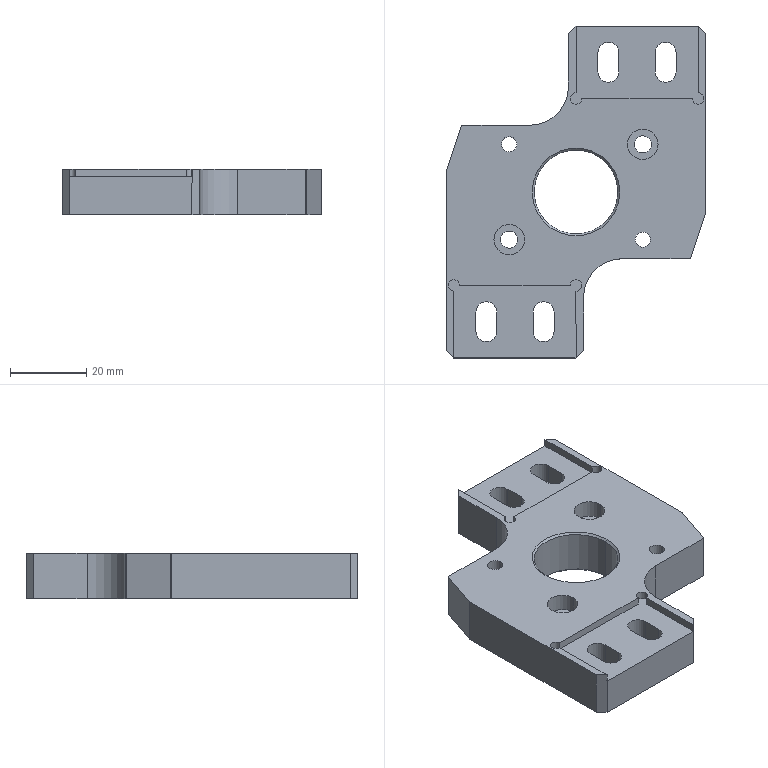Part | SolidWorks | features Chamfer 3, Cut 2, Fillet 2, ICE 2, Extrusion 1, HoleWzd 1 | 1 solid | 72 faces | box 68 x 87 x 12 mm | volume 40763 mm3 | cylinder 34 | plane 34 | cone 4 | commonest cylinder face diameters 5.5 x8 3 x6 1 x4 4 x4 4.5 x4 8 x4